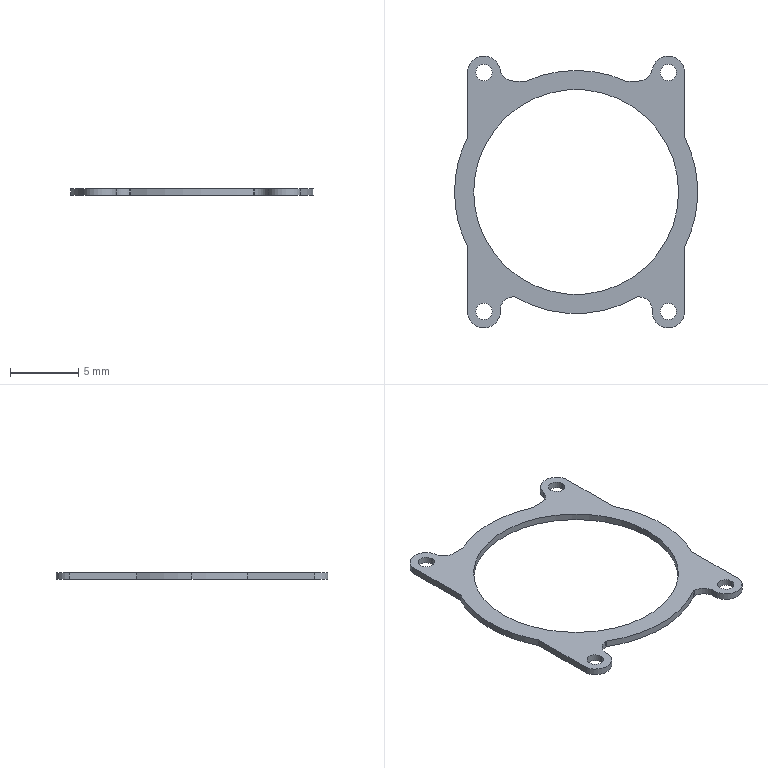Part | SolidWorks | features BaseBody 1, Scale 1 | 1 solid | 35 faces | box 17.8 x 19.9 x 0.5 mm | volume 54.481 mm3 | cylinder 23 | plane 12 | commonest cylinder face diameters 1.2 x8 17.8 x5 2 x4 2.4 x4 15 x2
STEP:
#1=CARTESIAN_POINT('',(7.5,23.098,0.75));
#2=VERTEX_POINT('',#1);
#3=CARTESIAN_POINT('',(-7.5,23.098,0.75));
#4=VERTEX_POINT('',#3);
#5=CARTESIAN_POINT('',(0.,23.098,0.75));
#6=DIRECTION('',(0.,0.,-1.));
#7=DIRECTION('',(-1.,0.,0.));
#8=AXIS2_PLACEMENT_3D('',#5,#6,#7);
#9=CIRCLE('',#8,7.5);
#10=EDGE_CURVE('',#2,#4,#9,.T.);
#11=ORIENTED_EDGE('',*,*,#10,.F.);
#12=CARTESIAN_POINT('',(7.5,23.098,0.25));
#13=VERTEX_POINT('',#12);
#14=CARTESIAN_POINT('',(7.5,23.098,0.75));
#15=DIRECTION('',(0.,0.,-1.));
#16=VECTOR('',#15,1000.);
#17=LINE('',#14,#16);
#18=EDGE_CURVE('',#2,#13,#17,.T.);
#19=ORIENTED_EDGE('',*,*,#18,.T.);
#20=CARTESIAN_POINT('',(-7.5,23.098,0.25));
#21=VERTEX_POINT('',#20);
#22=CARTESIAN_POINT('',(0.,23.098,0.25));
#23=DIRECTION('',(0.,0.,-1.));
#24=DIRECTION('',(-1.,0.,0.));
#25=AXIS2_PLACEMENT_3D('',#22,#23,#24);
#26=CIRCLE('',#25,7.5);
#27=EDGE_CURVE('',#13,#21,#26,.T.);
#28=ORIENTED_EDGE('',*,*,#27,.T.);
#29=CARTESIAN_POINT('',(-7.5,23.098,0.75));
#30=DIRECTION('',(0.,0.,-1.));
#31=VECTOR('',#30,1000.);
#32=LINE('',#29,#31);
#33=EDGE_CURVE('',#4,#21,#32,.T.);
#34=ORIENTED_EDGE('',*,*,#33,.F.);
#35=EDGE_LOOP('',(#11,#19,#28,#34));
#36=FACE_OUTER_BOUND('',#35,.T.);
#37=CARTESIAN_POINT('',(0.,23.098,0.75));
#38=DIRECTION('',(0.,0.,-1.));
#39=DIRECTION('',(-1.,0.,0.));
#40=AXIS2_PLACEMENT_3D('',#37,#38,#39);
#41=CYLINDRICAL_SURFACE('',#40,7.5);
#42=ADVANCED_FACE('',(#36),#41,.F.);
#43=CARTESIAN_POINT('',(-7.926,19.049,0.75));
#44=VERTEX_POINT('',#43);
#45=CARTESIAN_POINT('',(-8.9,23.098,0.75));
#46=VERTEX_POINT('',#45);
#47=CARTESIAN_POINT('',(0.,23.098,0.75));
#48=DIRECTION('',(0.,0.,-1.));
#49=DIRECTION('',(-1.,0.,0.));
#50=AXIS2_PLACEMENT_3D('',#47,#48,#49);
#51=CIRCLE('',#50,8.9);
#52=EDGE_CURVE('',#44,#46,#51,.T.);
#53=ORIENTED_EDGE('',*,*,#52,.T.);
#54=CARTESIAN_POINT('',(-8.9,23.098,0.25));
#55=VERTEX_POINT('',#54);
#56=CARTESIAN_POINT('',(-8.9,23.098,0.75));
#57=DIRECTION('',(0.,0.,-1.));
#58=VECTOR('',#57,1000.);
#59=LINE('',#56,#58);
#60=EDGE_CURVE('',#46,#55,#59,.T.);
#61=ORIENTED_EDGE('',*,*,#60,.T.);
#62=CARTESIAN_POINT('',(-7.926,19.049,0.25));
#63=VERTEX_POINT('',#62);
#64=CARTESIAN_POINT('',(0.,23.098,0.25));
#65=DIRECTION('',(0.,0.,1.));
#66=DIRECTION('',(-1.,0.,0.));
#67=AXIS2_PLACEMENT_3D('',#64,#65,#66);
#68=CIRCLE('',#67,8.9);
#69=EDGE_CURVE('',#55,#63,#68,.T.);
#70=ORIENTED_EDGE('',*,*,#69,.T.);
#71=CARTESIAN_POINT('',(-7.926,19.049,0.75));
#72=DIRECTION('',(0.,0.,1.));
#73=VECTOR('',#72,1000.);
#74=LINE('',#71,#73);
#75=EDGE_CURVE('',#63,#44,#74,.T.);
#76=ORIENTED_EDGE('',*,*,#75,.T.);
#77=EDGE_LOOP('',(#53,#61,#70,#76));
#78=FACE_OUTER_BOUND('',#77,.T.);
#79=CARTESIAN_POINT('',(0.,23.098,0.75));
#80=DIRECTION('',(0.,0.,-1.));
#81=DIRECTION('',(-1.,0.,0.));
#82=AXIS2_PLACEMENT_3D('',#79,#80,#81);
#83=CYLINDRICAL_SURFACE('',#82,8.9);
#84=ADVANCED_FACE('',(#78),#83,.T.);
#85=CARTESIAN_POINT('',(-6.15,14.348,0.25));
#86=VERTEX_POINT('',#85);
#87=CARTESIAN_POINT('',(-7.35,14.348,0.25));
#88=VERTEX_POINT('',#87);
#89=CARTESIAN_POINT('',(-6.75,14.348,0.25));
#90=DIRECTION('',(0.,0.,-1.));
#91=DIRECTION('',(1.,0.,0.));
#92=AXIS2_PLACEMENT_3D('',#89,#90,#91);
#93=CIRCLE('',#92,0.6);
#94=EDGE_CURVE('',#86,#88,#93,.T.);
#95=ORIENTED_EDGE('',*,*,#94,.T.);
#96=CARTESIAN_POINT('',(-7.35,14.348,0.75));
#97=VERTEX_POINT('',#96);
#98=CARTESIAN_POINT('',(-7.35,14.348,0.75));
#99=DIRECTION('',(0.,0.,1.));
#100=VECTOR('',#99,1000.);
#101=LINE('',#98,#100);
#102=EDGE_CURVE('',#88,#97,#101,.T.);
#103=ORIENTED_EDGE('',*,*,#102,.T.);
#104=CARTESIAN_POINT('',(-6.15,14.348,0.75));
#105=VERTEX_POINT('',#104);
#106=CARTESIAN_POINT('',(-6.75,14.348,0.75));
#107=DIRECTION('',(0.,0.,-1.));
#108=DIRECTION('',(1.,0.,0.));
#109=AXIS2_PLACEMENT_3D('',#106,#107,#108);
#110=CIRCLE('',#109,0.6);
#111=EDGE_CURVE('',#105,#97,#110,.T.);
#112=ORIENTED_EDGE('',*,*,#111,.F.);
#113=CARTESIAN_POINT('',(-6.15,14.348,0.75));
#114=DIRECTION('',(0.,0.,1.));
#115=VECTOR('',#114,1000.);
#116=LINE('',#113,#115);
#117=EDGE_CURVE('',#86,#105,#116,.T.);
#118=ORIENTED_EDGE('',*,*,#117,.F.);
#119=EDGE_LOOP('',(#95,#103,#112,#118));
#120=FACE_OUTER_BOUND('',#119,.T.);
#121=CARTESIAN_POINT('',(-6.75,14.348,0.75));
#122=DIRECTION('',(0.,0.,1.));
#123=DIRECTION('',(1.,0.,0.));
#124=AXIS2_PLACEMENT_3D('',#121,#122,#123);
#125=CYLINDRICAL_SURFACE('',#124,0.6);
#126=ADVANCED_FACE('',(#120),#125,.F.);
#127=CARTESIAN_POINT('',(7.35,14.348,0.25));
#128=VERTEX_POINT('',#127);
#129=CARTESIAN_POINT('',(6.15,14.348,0.25));
#130=VERTEX_POINT('',#129);
#131=CARTESIAN_POINT('',(6.75,14.348,0.25));
#132=DIRECTION('',(0.,0.,-1.));
#133=DIRECTION('',(1.,0.,0.));
#134=AXIS2_PLACEMENT_3D('',#131,#132,#133);
#135=CIRCLE('',#134,0.6);
#136=EDGE_CURVE('',#128,#130,#135,.T.);
#137=ORIENTED_EDGE('',*,*,#136,.T.);
#138=CARTESIAN_POINT('',(6.15,14.348,0.75));
#139=VERTEX_POINT('',#138);
#140=CARTESIAN_POINT('',(6.15,14.348,0.75));
#141=DIRECTION('',(0.,0.,1.));
#142=VECTOR('',#141,1000.);
#143=LINE('',#140,#142);
#144=EDGE_CURVE('',#130,#139,#143,.T.);
#145=ORIENTED_EDGE('',*,*,#144,.T.);
#146=CARTESIAN_POINT('',(7.35,14.348,0.75));
#147=VERTEX_POINT('',#146);
#148=CARTESIAN_POINT('',(6.75,14.348,0.75));
#149=DIRECTION('',(0.,0.,-1.));
#150=DIRECTION('',(1.,0.,0.));
#151=AXIS2_PLACEMENT_3D('',#148,#149,#150);
#152=CIRCLE('',#151,0.6);
#153=EDGE_CURVE('',#147,#139,#152,.T.);
#154=ORIENTED_EDGE('',*,*,#153,.F.);
#155=CARTESIAN_POINT('',(7.35,14.348,0.75));
#156=DIRECTION('',(0.,0.,1.));
#157=VECTOR('',#156,1000.);
#158=LINE('',#155,#157);
#159=EDGE_CURVE('',#128,#147,#158,.T.);
#160=ORIENTED_EDGE('',*,*,#159,.F.);
#161=EDGE_LOOP('',(#137,#145,#154,#160));
#162=FACE_OUTER_BOUND('',#161,.T.);
#163=CARTESIAN_POINT('',(6.75,14.348,0.75));
#164=DIRECTION('',(0.,0.,1.));
#165=DIRECTION('',(1.,0.,0.));
#166=AXIS2_PLACEMENT_3D('',#163,#164,#165);
#167=CYLINDRICAL_SURFACE('',#166,0.6);
#168=ADVANCED_FACE('',(#162),#167,.F.);
#169=CARTESIAN_POINT('',(7.35,31.848,0.25));
#170=VERTEX_POINT('',#169);
#171=CARTESIAN_POINT('',(6.15,31.848,0.25));
#172=VERTEX_POINT('',#171);
#173=CARTESIAN_POINT('',(6.75,31.848,0.25));
#174=DIRECTION('',(0.,0.,-1.));
#175=DIRECTION('',(1.,0.,0.));
#176=AXIS2_PLACEMENT_3D('',#173,#174,#175);
#177=CIRCLE('',#176,0.6);
#178=EDGE_CURVE('',#170,#172,#177,.T.);
#179=ORIENTED_EDGE('',*,*,#178,.T.);
#180=CARTESIAN_POINT('',(6.15,31.848,0.75));
#181=VERTEX_POINT('',#180);
#182=CARTESIAN_POINT('',(6.15,31.848,0.75));
#183=DIRECTION('',(0.,0.,1.));
#184=VECTOR('',#183,1000.);
#185=LINE('',#182,#184);
#186=EDGE_CURVE('',#172,#181,#185,.T.);
#187=ORIENTED_EDGE('',*,*,#186,.T.);
#188=CARTESIAN_POINT('',(7.35,31.848,0.75));
#189=VERTEX_POINT('',#188);
#190=CARTESIAN_POINT('',(6.75,31.848,0.75));
#191=DIRECTION('',(0.,0.,-1.));
#192=DIRECTION('',(1.,0.,0.));
#193=AXIS2_PLACEMENT_3D('',#190,#191,#192);
#194=CIRCLE('',#193,0.6);
#195=EDGE_CURVE('',#189,#181,#194,.T.);
#196=ORIENTED_EDGE('',*,*,#195,.F.);
#197=CARTESIAN_POINT('',(7.35,31.848,0.75));
#198=DIRECTION('',(0.,0.,1.));
#199=VECTOR('',#198,1000.);
#200=LINE('',#197,#199);
#201=EDGE_CURVE('',#170,#189,#200,.T.);
#202=ORIENTED_EDGE('',*,*,#201,.F.);
#203=EDGE_LOOP('',(#179,#187,#196,#202));
#204=FACE_OUTER_BOUND('',#203,.T.);
#205=CARTESIAN_POINT('',(6.75,31.848,0.75));
#206=DIRECTION('',(0.,0.,1.));
#207=DIRECTION('',(1.,0.,0.));
#208=AXIS2_PLACEMENT_3D('',#205,#206,#207);
#209=CYLINDRICAL_SURFACE('',#208,0.6);
#210=ADVANCED_FACE('',(#204),#209,.F.);
#211=CARTESIAN_POINT('',(-6.15,31.848,0.25));
#212=VERTEX_POINT('',#211);
#213=CARTESIAN_POINT('',(-7.35,31.848,0.25));
#214=VERTEX_POINT('',#213);
#215=CARTESIAN_POINT('',(-6.75,31.848,0.25));
#216=DIRECTION('',(0.,0.,-1.));
#217=DIRECTION('',(1.,0.,0.));
#218=AXIS2_PLACEMENT_3D('',#215,#216,#217);
#219=CIRCLE('',#218,0.6);
#220=EDGE_CURVE('',#212,#214,#219,.T.);
#221=ORIENTED_EDGE('',*,*,#220,.T.);
#222=CARTESIAN_POINT('',(-7.35,31.848,0.75));
#223=VERTEX_POINT('',#222);
#224=CARTESIAN_POINT('',(-7.35,31.848,0.75));
#225=DIRECTION('',(0.,0.,1.));
#226=VECTOR('',#225,1000.);
#227=LINE('',#224,#226);
#228=EDGE_CURVE('',#214,#223,#227,.T.);
#229=ORIENTED_EDGE('',*,*,#228,.T.);
#230=CARTESIAN_POINT('',(-6.15,31.848,0.75));
#231=VERTEX_POINT('',#230);
#232=CARTESIAN_POINT('',(-6.75,31.848,0.75));
#233=DIRECTION('',(0.,0.,-1.));
#234=DIRECTION('',(1.,0.,0.));
#235=AXIS2_PLACEMENT_3D('',#232,#233,#234);
#236=CIRCLE('',#235,0.6);
#237=EDGE_CURVE('',#231,#223,#236,.T.);
#238=ORIENTED_EDGE('',*,*,#237,.F.);
#239=CARTESIAN_POINT('',(-6.15,31.848,0.75));
#240=DIRECTION('',(0.,0.,1.));
#241=VECTOR('',#240,1000.);
#242=LINE('',#239,#241);
#243=EDGE_CURVE('',#212,#231,#242,.T.);
#244=ORIENTED_EDGE('',*,*,#243,.F.);
#245=EDGE_LOOP('',(#221,#229,#238,#244));
#246=FACE_OUTER_BOUND('',#245,.T.);
#247=CARTESIAN_POINT('',(-6.75,31.848,0.75));
#248=DIRECTION('',(0.,0.,1.));
#249=DIRECTION('',(1.,0.,0.));
#250=AXIS2_PLACEMENT_3D('',#247,#248,#249);
#251=CYLINDRICAL_SURFACE('',#250,0.6);
#252=ADVANCED_FACE('',(#246),#251,.F.);
#253=CARTESIAN_POINT('',(0.,23.098,0.25));
#254=DIRECTION('',(0.,0.,-1.));
#255=DIRECTION('',(-1.,0.,0.));
#256=AXIS2_PLACEMENT_3D('',#253,#254,#255);
#257=CIRCLE('',#256,7.5);
#258=EDGE_CURVE('',#21,#13,#257,.T.);
#259=ORIENTED_EDGE('',*,*,#258,.F.);
#260=ORIENTED_EDGE('',*,*,#27,.F.);
#261=EDGE_LOOP('',(#259,#260));
#262=FACE_BOUND('',#261,.T.);
#263=CARTESIAN_POINT('',(-7.926,32.088,0.25));
#264=VERTEX_POINT('',#263);
#265=CARTESIAN_POINT('',(-7.926,27.146,0.25));
#266=VERTEX_POINT('',#265);
#267=CARTESIAN_POINT('',(-7.926,23.098,0.25));
#268=DIRECTION('',(0.,-1.,0.));
#269=VECTOR('',#268,1000.);
#270=LINE('',#267,#269);
#271=EDGE_CURVE('',#264,#266,#270,.T.);
#272=ORIENTED_EDGE('',*,*,#271,.F.);
#273=CARTESIAN_POINT('',(-5.574,32.088,0.25));
#274=VERTEX_POINT('',#273);
#275=CARTESIAN_POINT('',(-6.75,31.848,0.25));
#276=DIRECTION('',(0.,0.,1.));
#277=DIRECTION('',(-1.,0.,0.));
#278=AXIS2_PLACEMENT_3D('',#275,#276,#277);
#279=CIRCLE('',#278,1.2);
#280=EDGE_CURVE('',#274,#264,#279,.T.);
#281=ORIENTED_EDGE('',*,*,#280,.F.);
#282=CARTESIAN_POINT('',(-4.583,31.223,0.25));
#283=VERTEX_POINT('',#282);
#284=CARTESIAN_POINT('',(-4.583,32.223,0.25));
#285=DIRECTION('',(0.,0.,-1.));
#286=DIRECTION('',(-1.,0.,0.));
#287=AXIS2_PLACEMENT_3D('',#284,#285,#286);
#288=CIRCLE('',#287,1.);
#289=EDGE_CURVE('',#283,#274,#288,.T.);
#290=ORIENTED_EDGE('',*,*,#289,.F.);
#291=CARTESIAN_POINT('',(-3.632,31.223,0.25));
#292=VERTEX_POINT('',#291);
#293=CARTESIAN_POINT('',(0.,31.223,0.25));
#294=DIRECTION('',(-1.,0.,0.));
#295=VECTOR('',#294,1000.);
#296=LINE('',#293,#295);
#297=EDGE_CURVE('',#292,#283,#296,.T.);
#298=ORIENTED_EDGE('',*,*,#297,.F.);
#299=CARTESIAN_POINT('',(3.632,31.223,0.25));
#300=VERTEX_POINT('',#299);
#301=CARTESIAN_POINT('',(0.,23.098,0.25));
#302=DIRECTION('',(0.,0.,1.));
#303=DIRECTION('',(-1.,0.,0.));
#304=AXIS2_PLACEMENT_3D('',#301,#302,#303);
#305=CIRCLE('',#304,8.9);
#306=EDGE_CURVE('',#300,#292,#305,.T.);
#307=ORIENTED_EDGE('',*,*,#306,.F.);
#308=CARTESIAN_POINT('',(4.583,31.223,0.25));
#309=VERTEX_POINT('',#308);
#310=CARTESIAN_POINT('',(0.,31.223,0.25));
#311=DIRECTION('',(-1.,0.,0.));
#312=VECTOR('',#311,1000.);
#313=LINE('',#310,#312);
#314=EDGE_CURVE('',#309,#300,#313,.T.);
#315=ORIENTED_EDGE('',*,*,#314,.F.);
#316=CARTESIAN_POINT('',(5.574,32.088,0.25));
#317=VERTEX_POINT('',#316);
#318=CARTESIAN_POINT('',(4.583,32.223,0.25));
#319=DIRECTION('',(0.,0.,-1.));
#320=DIRECTION('',(-1.,0.,0.));
#321=AXIS2_PLACEMENT_3D('',#318,#319,#320);
#322=CIRCLE('',#321,1.);
#323=EDGE_CURVE('',#317,#309,#322,.T.);
#324=ORIENTED_EDGE('',*,*,#323,.F.);
#325=CARTESIAN_POINT('',(7.926,32.088,0.25));
#326=VERTEX_POINT('',#325);
#327=CARTESIAN_POINT('',(6.75,31.848,0.25));
#328=DIRECTION('',(0.,0.,1.));
#329=DIRECTION('',(-1.,0.,0.));
#330=AXIS2_PLACEMENT_3D('',#327,#328,#329);
#331=CIRCLE('',#330,1.2);
#332=EDGE_CURVE('',#326,#317,#331,.T.);
#333=ORIENTED_EDGE('',*,*,#332,.F.);
#334=CARTESIAN_POINT('',(7.926,27.146,0.25));
#335=VERTEX_POINT('',#334);
#336=CARTESIAN_POINT('',(7.926,23.098,0.25));
#337=DIRECTION('',(0.,1.,0.));
#338=VECTOR('',#337,1000.);
#339=LINE('',#336,#338);
#340=EDGE_CURVE('',#335,#326,#339,.T.);
#341=ORIENTED_EDGE('',*,*,#340,.F.);
#342=CARTESIAN_POINT('',(7.926,19.049,0.25));
#343=VERTEX_POINT('',#342);
#344=CARTESIAN_POINT('',(0.,23.098,0.25));
#345=DIRECTION('',(0.,0.,1.));
#346=DIRECTION('',(-1.,0.,0.));
#347=AXIS2_PLACEMENT_3D('',#344,#345,#346);
#348=CIRCLE('',#347,8.9);
#349=EDGE_CURVE('',#343,#335,#348,.T.);
#350=ORIENTED_EDGE('',*,*,#349,.F.);
#351=CARTESIAN_POINT('',(7.926,14.108,0.25));
#352=VERTEX_POINT('',#351);
#353=CARTESIAN_POINT('',(7.926,23.098,0.25));
#354=DIRECTION('',(0.,1.,0.));
#355=VECTOR('',#354,1000.);
#356=LINE('',#353,#355);
#357=EDGE_CURVE('',#352,#343,#356,.T.);
#358=ORIENTED_EDGE('',*,*,#357,.F.);
#359=CARTESIAN_POINT('',(5.574,14.108,0.25));
#360=VERTEX_POINT('',#359);
#361=CARTESIAN_POINT('',(6.75,14.348,0.25));
#362=DIRECTION('',(0.,0.,1.));
#363=DIRECTION('',(-1.,0.,0.));
#364=AXIS2_PLACEMENT_3D('',#361,#362,#363);
#365=CIRCLE('',#364,1.2);
#366=EDGE_CURVE('',#360,#352,#365,.T.);
#367=ORIENTED_EDGE('',*,*,#366,.F.);
#368=CARTESIAN_POINT('',(5.574,14.423,0.25));
#369=VERTEX_POINT('',#368);
#370=CARTESIAN_POINT('',(5.574,23.098,0.25));
#371=DIRECTION('',(0.,-1.,0.));
#372=VECTOR('',#371,1000.);
#373=LINE('',#370,#372);
#374=EDGE_CURVE('',#369,#360,#373,.T.);
#375=ORIENTED_EDGE('',*,*,#374,.F.);
#376=CARTESIAN_POINT('',(4.574,15.423,0.25));
#377=VERTEX_POINT('',#376);
#378=CARTESIAN_POINT('',(4.574,14.423,0.25));
#379=DIRECTION('',(0.,0.,-1.));
#380=DIRECTION('',(1.,0.,0.));
#381=AXIS2_PLACEMENT_3D('',#378,#379,#380);
#382=CIRCLE('',#381,1.);
#383=EDGE_CURVE('',#377,#369,#382,.T.);
#384=ORIENTED_EDGE('',*,*,#383,.F.);
#385=CARTESIAN_POINT('',(4.506,15.423,0.25));
#386=VERTEX_POINT('',#385);
#387=CARTESIAN_POINT('',(0.,15.423,0.25));
#388=DIRECTION('',(1.,0.,0.));
#389=VECTOR('',#388,1000.);
#390=LINE('',#387,#389);
#391=EDGE_CURVE('',#386,#377,#390,.T.);
#392=ORIENTED_EDGE('',*,*,#391,.F.);
#393=CARTESIAN_POINT('',(-4.506,15.423,0.25));
#394=VERTEX_POINT('',#393);
#395=CARTESIAN_POINT('',(0.,23.098,0.25));
#396=DIRECTION('',(0.,0.,1.));
#397=DIRECTION('',(-1.,0.,0.));
#398=AXIS2_PLACEMENT_3D('',#395,#396,#397);
#399=CIRCLE('',#398,8.9);
#400=EDGE_CURVE('',#394,#386,#399,.T.);
#401=ORIENTED_EDGE('',*,*,#400,.F.);
#402=CARTESIAN_POINT('',(-4.574,15.423,0.25));
#403=VERTEX_POINT('',#402);
#404=CARTESIAN_POINT('',(0.,15.423,0.25));
#405=DIRECTION('',(1.,0.,0.));
#406=VECTOR('',#405,1000.);
#407=LINE('',#404,#406);
#408=EDGE_CURVE('',#403,#394,#407,.T.);
#409=ORIENTED_EDGE('',*,*,#408,.F.);
#410=CARTESIAN_POINT('',(-5.574,14.423,0.25));
#411=VERTEX_POINT('',#410);
#412=CARTESIAN_POINT('',(-4.574,14.423,0.25));
#413=DIRECTION('',(0.,0.,-1.));
#414=DIRECTION('',(1.,0.,0.));
#415=AXIS2_PLACEMENT_3D('',#412,#413,#414);
#416=CIRCLE('',#415,1.);
#417=EDGE_CURVE('',#411,#403,#416,.T.);
#418=ORIENTED_EDGE('',*,*,#417,.F.);
#419=CARTESIAN_POINT('',(-5.574,14.108,0.25));
#420=VERTEX_POINT('',#419);
#421=CARTESIAN_POINT('',(-5.574,23.098,0.25));
#422=DIRECTION('',(0.,1.,0.));
#423=VECTOR('',#422,1000.);
#424=LINE('',#421,#423);
#425=EDGE_CURVE('',#420,#411,#424,.T.);
#426=ORIENTED_EDGE('',*,*,#425,.F.);
#427=CARTESIAN_POINT('',(-7.926,14.108,0.25));
#428=VERTEX_POINT('',#427);
#429=CARTESIAN_POINT('',(-6.75,14.348,0.25));
#430=DIRECTION('',(0.,0.,1.));
#431=DIRECTION('',(-1.,0.,0.));
#432=AXIS2_PLACEMENT_3D('',#429,#430,#431);
#433=CIRCLE('',#432,1.2);
#434=EDGE_CURVE('',#428,#420,#433,.T.);
#435=ORIENTED_EDGE('',*,*,#434,.F.);
#436=CARTESIAN_POINT('',(-7.926,23.098,0.25));
#437=DIRECTION('',(0.,-1.,0.));
#438=VECTOR('',#437,1000.);
#439=LINE('',#436,#438);
#440=EDGE_CURVE('',#63,#428,#439,.T.);
#441=ORIENTED_EDGE('',*,*,#440,.F.);
#442=ORIENTED_EDGE('',*,*,#69,.F.);
#443=CARTESIAN_POINT('',(0.,23.098,0.25));
#444=DIRECTION('',(0.,0.,1.));
#445=DIRECTION('',(-1.,0.,0.));
#446=AXIS2_PLACEMENT_3D('',#443,#444,#445);
#447=CIRCLE('',#446,8.9);
#448=EDGE_CURVE('',#266,#55,#447,.T.);
#449=ORIENTED_EDGE('',*,*,#448,.F.);
#450=EDGE_LOOP('',(#272,#281,#290,#298,#307,#315,#324,#333,#341,#350,#358,#367,#375,#384,#392,#401,#409,#418,#426,#435,#441,#442,#449));
#451=FACE_OUTER_BOUND('',#450,.T.);
#452=ORIENTED_EDGE('',*,*,#94,.F.);
#453=CARTESIAN_POINT('',(-6.75,14.348,0.25));
#454=DIRECTION('',(0.,0.,-1.));
#455=DIRECTION('',(1.,0.,0.));
#456=AXIS2_PLACEMENT_3D('',#453,#454,#455);
#457=CIRCLE('',#456,0.6);
#458=EDGE_CURVE('',#88,#86,#457,.T.);
#459=ORIENTED_EDGE('',*,*,#458,.F.);
#460=EDGE_LOOP('',(#452,#459));
#461=FACE_BOUND('',#460,.T.);
#462=ORIENTED_EDGE('',*,*,#136,.F.);
#463=CARTESIAN_POINT('',(6.75,14.348,0.25));
#464=DIRECTION('',(0.,0.,-1.));
#465=DIRECTION('',(1.,0.,0.));
#466=AXIS2_PLACEMENT_3D('',#463,#464,#465);
#467=CIRCLE('',#466,0.6);
#468=EDGE_CURVE('',#130,#128,#467,.T.);
#469=ORIENTED_EDGE('',*,*,#468,.F.);
#470=EDGE_LOOP('',(#462,#469));
#471=FACE_BOUND('',#470,.T.);
#472=ORIENTED_EDGE('',*,*,#178,.F.);
#473=CARTESIAN_POINT('',(6.75,31.848,0.25));
#474=DIRECTION('',(0.,0.,-1.));
#475=DIRECTION('',(1.,0.,0.));
#476=AXIS2_PLACEMENT_3D('',#473,#474,#475);
#477=CIRCLE('',#476,0.6);
#478=EDGE_CURVE('',#172,#170,#477,.T.);
#479=ORIENTED_EDGE('',*,*,#478,.F.);
#480=EDGE_LOOP('',(#472,#479));
#481=FACE_BOUND('',#480,.T.);
#482=ORIENTED_EDGE('',*,*,#220,.F.);
#483=CARTESIAN_POINT('',(-6.75,31.848,0.25));
#484=DIRECTION('',(0.,0.,-1.));
#485=DIRECTION('',(1.,0.,0.));
#486=AXIS2_PLACEMENT_3D('',#483,#484,#485);
#487=CIRCLE('',#486,0.6);
#488=EDGE_CURVE('',#214,#212,#487,.T.);
#489=ORIENTED_EDGE('',*,*,#488,.F.);
#490=EDGE_LOOP('',(#482,#489));
#491=FACE_BOUND('',#490,.T.);
#492=CARTESIAN_POINT('',(0.,23.098,0.25));
#493=DIRECTION('',(0.,0.,1.));
#494=DIRECTION('',(1.,0.,0.));
#495=AXIS2_PLACEMENT_3D('',#492,#493,#494);
#496=PLANE('',#495);
#497=ADVANCED_FACE('',(#262,#451,#461,#471,#481,#491),#496,.F.);
#498=ORIENTED_EDGE('',*,*,#18,.F.);
#499=CARTESIAN_POINT('',(0.,23.098,0.75));
#500=DIRECTION('',(0.,0.,-1.));
#501=DIRECTION('',(-1.,0.,0.));
#502=AXIS2_PLACEMENT_3D('',#499,#500,#501);
#503=CIRCLE('',#502,7.5);
#504=EDGE_CURVE('',#4,#2,#503,.T.);
#505=ORIENTED_EDGE('',*,*,#504,.F.);
#506=ORIENTED_EDGE('',*,*,#33,.T.);
#507=ORIENTED_EDGE('',*,*,#258,.T.);
#508=EDGE_LOOP('',(#498,#505,#506,#507));
#509=FACE_OUTER_BOUND('',#508,.T.);
#510=CARTESIAN_POINT('',(0.,23.098,0.75));
#511=DIRECTION('',(0.,0.,-1.));
#512=DIRECTION('',(-1.,0.,0.));
#513=AXIS2_PLACEMENT_3D('',#510,#511,#512);
#514=CYLINDRICAL_SURFACE('',#513,7.5);
#515=ADVANCED_FACE('',(#509),#514,.F.);
#516=ORIENTED_EDGE('',*,*,#60,.F.);
#517=CARTESIAN_POINT('',(-7.926,27.146,0.75));
#518=VERTEX_POINT('',#517);
#519=CARTESIAN_POINT('',(0.,23.098,0.75));
#520=DIRECTION('',(0.,0.,-1.));
#521=DIRECTION('',(-1.,0.,0.));
#522=AXIS2_PLACEMENT_3D('',#519,#520,#521);
#523=CIRCLE('',#522,8.9);
#524=EDGE_CURVE('',#46,#518,#523,.T.);
#525=ORIENTED_EDGE('',*,*,#524,.T.);
#526=CARTESIAN_POINT('',(-7.926,27.146,0.75));
#527=DIRECTION('',(0.,0.,-1.));
#528=VECTOR('',#527,1000.);
#529=LINE('',#526,#528);
#530=EDGE_CURVE('',#518,#266,#529,.T.);
#531=ORIENTED_EDGE('',*,*,#530,.T.);
#532=ORIENTED_EDGE('',*,*,#448,.T.);
#533=EDGE_LOOP('',(#516,#525,#531,#532));
#534=FACE_OUTER_BOUND('',#533,.T.);
#535=CARTESIAN_POINT('',(0.,23.098,0.75));
#536=DIRECTION('',(0.,0.,-1.));
#537=DIRECTION('',(-1.,0.,0.));
#538=AXIS2_PLACEMENT_3D('',#535,#536,#537);
#539=CYLINDRICAL_SURFACE('',#538,8.9);
#540=ADVANCED_FACE('',(#534),#539,.T.);
#541=ORIENTED_EDGE('',*,*,#530,.F.);
#542=CARTESIAN_POINT('',(-7.926,32.088,0.75));
#543=VERTEX_POINT('',#542);
#544=CARTESIAN_POINT('',(-7.926,32.088,0.75));
#545=DIRECTION('',(0.,-1.,0.));
#546=VECTOR('',#545,1000.);
#547=LINE('',#544,#546);
#548=EDGE_CURVE('',#543,#518,#547,.T.);
#549=ORIENTED_EDGE('',*,*,#548,.F.);
#550=CARTESIAN_POINT('',(-7.926,32.088,0.75));
#551=DIRECTION('',(0.,0.,1.));
#552=VECTOR('',#551,1000.);
#553=LINE('',#550,#552);
#554=EDGE_CURVE('',#264,#543,#553,.T.);
#555=ORIENTED_EDGE('',*,*,#554,.F.);
#556=ORIENTED_EDGE('',*,*,#271,.T.);
#557=EDGE_LOOP('',(#541,#549,#555,#556));
#558=FACE_OUTER_BOUND('',#557,.T.);
#559=CARTESIAN_POINT('',(-7.926,32.088,0.75));
#560=DIRECTION('',(1.,0.,0.));
#561=DIRECTION('',(0.,1.,0.));
#562=AXIS2_PLACEMENT_3D('',#559,#560,#561);
#563=PLANE('',#562);
#564=ADVANCED_FACE('',(#558),#563,.F.);
#565=CARTESIAN_POINT('',(-5.574,32.088,0.75));
#566=VERTEX_POINT('',#565);
#567=CARTESIAN_POINT('',(-6.75,31.848,0.75));
#568=DIRECTION('',(0.,0.,-1.));
#569=DIRECTION('',(-1.,0.,0.));
#570=AXIS2_PLACEMENT_3D('',#567,#568,#569);
#571=CIRCLE('',#570,1.2);
#572=EDGE_CURVE('',#543,#566,#571,.T.);
#573=ORIENTED_EDGE('',*,*,#572,.T.);
#574=CARTESIAN_POINT('',(-5.574,32.088,0.75));
#575=DIRECTION('',(0.,0.,-1.));
#576=VECTOR('',#575,1000.);
#577=LINE('',#574,#576);
#578=EDGE_CURVE('',#566,#274,#577,.T.);
#579=ORIENTED_EDGE('',*,*,#578,.T.);
#580=ORIENTED_EDGE('',*,*,#280,.T.);
#581=ORIENTED_EDGE('',*,*,#554,.T.);
#582=EDGE_LOOP('',(#573,#579,#580,#581));
#583=FACE_OUTER_BOUND('',#582,.T.);
#584=CARTESIAN_POINT('',(-6.75,31.848,0.75));
#585=DIRECTION('',(0.,0.,-1.));
#586=DIRECTION('',(-1.,0.,0.));
#587=AXIS2_PLACEMENT_3D('',#584,#585,#586);
#588=CYLINDRICAL_SURFACE('',#587,1.2);
#589=ADVANCED_FACE('',(#583),#588,.T.);
#590=CARTESIAN_POINT('',(-4.583,31.223,0.75));
#591=VERTEX_POINT('',#590);
#592=CARTESIAN_POINT('',(-4.583,31.223,0.75));
#593=DIRECTION('',(0.,0.,1.));
#594=VECTOR('',#593,1000.);
#595=LINE('',#592,#594);
#596=EDGE_CURVE('',#283,#591,#595,.T.);
#597=ORIENTED_EDGE('',*,*,#596,.F.);
#598=ORIENTED_EDGE('',*,*,#289,.T.);
#599=ORIENTED_EDGE('',*,*,#578,.F.);
#600=CARTESIAN_POINT('',(-4.583,32.223,0.75));
#601=DIRECTION('',(0.,0.,-1.));
#602=DIRECTION('',(-1.,0.,0.));
#603=AXIS2_PLACEMENT_3D('',#600,#601,#602);
#604=CIRCLE('',#603,1.);
#605=EDGE_CURVE('',#591,#566,#604,.T.);
#606=ORIENTED_EDGE('',*,*,#605,.F.);
#607=EDGE_LOOP('',(#597,#598,#599,#606));
#608=FACE_OUTER_BOUND('',#607,.T.);
#609=CARTESIAN_POINT('',(-4.583,32.223,0.75));
#610=DIRECTION('',(0.,0.,-1.));
#611=DIRECTION('',(-1.,0.,0.));
#612=AXIS2_PLACEMENT_3D('',#609,#610,#611);
#613=CYLINDRICAL_SURFACE('',#612,1.);
#614=ADVANCED_FACE('',(#608),#613,.F.);
#615=ORIENTED_EDGE('',*,*,#596,.T.);
#616=CARTESIAN_POINT('',(-3.632,31.223,0.75));
#617=VERTEX_POINT('',#616);
#618=CARTESIAN_POINT('',(-3.632,31.223,0.75));
#619=DIRECTION('',(-1.,0.,0.));
#620=VECTOR('',#619,1000.);
#621=LINE('',#618,#620);
#622=EDGE_CURVE('',#617,#591,#621,.T.);
#623=ORIENTED_EDGE('',*,*,#622,.F.);
#624=CARTESIAN_POINT('',(-3.632,31.223,0.75));
#625=DIRECTION('',(0.,0.,1.));
#626=VECTOR('',#625,1000.);
#627=LINE('',#624,#626);
#628=EDGE_CURVE('',#292,#617,#627,.T.);
#629=ORIENTED_EDGE('',*,*,#628,.F.);
#630=ORIENTED_EDGE('',*,*,#297,.T.);
#631=EDGE_LOOP('',(#615,#623,#629,#630));
#632=FACE_OUTER_BOUND('',#631,.T.);
#633=CARTESIAN_POINT('',(-3.632,31.223,0.75));
#634=DIRECTION('',(0.,-1.,0.));
#635=DIRECTION('',(0.,0.,-1.));
#636=AXIS2_PLACEMENT_3D('',#633,#634,#635);
#637=PLANE('',#636);
#638=ADVANCED_FACE('',(#632),#637,.F.);
#639=CARTESIAN_POINT('',(3.632,31.223,0.75));
#640=VERTEX_POINT('',#639);
#641=CARTESIAN_POINT('',(0.,23.098,0.75));
#642=DIRECTION('',(0.,0.,-1.));
#643=DIRECTION('',(-1.,0.,0.));
#644=AXIS2_PLACEMENT_3D('',#641,#642,#643);
#645=CIRCLE('',#644,8.9);
#646=EDGE_CURVE('',#617,#640,#645,.T.);
#647=ORIENTED_EDGE('',*,*,#646,.T.);
#648=CARTESIAN_POINT('',(3.632,31.223,0.75));
#649=DIRECTION('',(0.,0.,-1.));
#650=VECTOR('',#649,1000.);
#651=LINE('',#648,#650);
#652=EDGE_CURVE('',#640,#300,#651,.T.);
#653=ORIENTED_EDGE('',*,*,#652,.T.);
#654=ORIENTED_EDGE('',*,*,#306,.T.);
#655=ORIENTED_EDGE('',*,*,#628,.T.);
#656=EDGE_LOOP('',(#647,#653,#654,#655));
#657=FACE_OUTER_BOUND('',#656,.T.);
#658=CARTESIAN_POINT('',(0.,23.098,0.75));
#659=DIRECTION('',(0.,0.,-1.));
#660=DIRECTION('',(-1.,0.,0.));
#661=AXIS2_PLACEMENT_3D('',#658,#659,#660);
#662=CYLINDRICAL_SURFACE('',#661,8.9);
#663=ADVANCED_FACE('',(#657),#662,.T.);
#664=CARTESIAN_POINT('',(4.583,31.223,0.75));
#665=VERTEX_POINT('',#664);
#666=CARTESIAN_POINT('',(4.583,31.223,0.75));
#667=DIRECTION('',(0.,0.,1.));
#668=VECTOR('',#667,1000.);
#669=LINE('',#666,#668);
#670=EDGE_CURVE('',#309,#665,#669,.T.);
#671=ORIENTED_EDGE('',*,*,#670,.F.);
#672=ORIENTED_EDGE('',*,*,#314,.T.);
#673=ORIENTED_EDGE('',*,*,#652,.F.);
#674=CARTESIAN_POINT('',(5.574,31.223,0.75));
#675=DIRECTION('',(-1.,0.,0.));
#676=VECTOR('',#675,1000.);
#677=LINE('',#674,#676);
#678=EDGE_CURVE('',#665,#640,#677,.T.);
#679=ORIENTED_EDGE('',*,*,#678,.F.);
#680=EDGE_LOOP('',(#671,#672,#673,#679));
#681=FACE_OUTER_BOUND('',#680,.T.);
#682=CARTESIAN_POINT('',(5.574,31.223,0.75));
#683=DIRECTION('',(0.,-1.,0.));
#684=DIRECTION('',(1.,0.,0.));
#685=AXIS2_PLACEMENT_3D('',#682,#683,#684);
#686=PLANE('',#685);
#687=ADVANCED_FACE('',(#681),#686,.F.);
#688=CARTESIAN_POINT('',(5.574,32.088,0.75));
#689=VERTEX_POINT('',#688);
#690=CARTESIAN_POINT('',(5.574,32.088,0.75));
#691=DIRECTION('',(0.,0.,1.));
#692=VECTOR('',#691,1000.);
#693=LINE('',#690,#692);
#694=EDGE_CURVE('',#317,#689,#693,.T.);
#695=ORIENTED_EDGE('',*,*,#694,.F.);
#696=ORIENTED_EDGE('',*,*,#323,.T.);
#697=ORIENTED_EDGE('',*,*,#670,.T.);
#698=CARTESIAN_POINT('',(4.583,32.223,0.75));
#699=DIRECTION('',(0.,0.,-1.));
#700=DIRECTION('',(-1.,0.,0.));
#701=AXIS2_PLACEMENT_3D('',#698,#699,#700);
#702=CIRCLE('',#701,1.);
#703=EDGE_CURVE('',#689,#665,#702,.T.);
#704=ORIENTED_EDGE('',*,*,#703,.F.);
#705=EDGE_LOOP('',(#695,#696,#697,#704));
#706=FACE_OUTER_BOUND('',#705,.T.);
#707=CARTESIAN_POINT('',(4.583,32.223,0.75));
#708=DIRECTION('',(0.,0.,-1.));
#709=DIRECTION('',(-1.,0.,0.));
#710=AXIS2_PLACEMENT_3D('',#707,#708,#709);
#711=CYLINDRICAL_SURFACE('',#710,1.);
#712=ADVANCED_FACE('',(#706),#711,.F.);
#713=CARTESIAN_POINT('',(7.926,32.088,0.75));
#714=VERTEX_POINT('',#713);
#715=CARTESIAN_POINT('',(6.75,31.848,0.75));
#716=DIRECTION('',(0.,0.,-1.));
#717=DIRECTION('',(-1.,0.,0.));
#718=AXIS2_PLACEMENT_3D('',#715,#716,#717);
#719=CIRCLE('',#718,1.2);
#720=EDGE_CURVE('',#689,#714,#719,.T.);
#721=ORIENTED_EDGE('',*,*,#720,.T.);
#722=CARTESIAN_POINT('',(7.926,32.088,0.75));
#723=DIRECTION('',(0.,0.,-1.));
#724=VECTOR('',#723,1000.);
#725=LINE('',#722,#724);
#726=EDGE_CURVE('',#714,#326,#725,.T.);
#727=ORIENTED_EDGE('',*,*,#726,.T.);
#728=ORIENTED_EDGE('',*,*,#332,.T.);
#729=ORIENTED_EDGE('',*,*,#694,.T.);
#730=EDGE_LOOP('',(#721,#727,#728,#729));
#731=FACE_OUTER_BOUND('',#730,.T.);
#732=CARTESIAN_POINT('',(6.75,31.848,0.75));
#733=DIRECTION('',(0.,0.,-1.));
#734=DIRECTION('',(-1.,0.,0.));
#735=AXIS2_PLACEMENT_3D('',#732,#733,#734);
#736=CYLINDRICAL_SURFACE('',#735,1.2);
#737=ADVANCED_FACE('',(#731),#736,.T.);
#738=ORIENTED_EDGE('',*,*,#726,.F.);
#739=CARTESIAN_POINT('',(7.926,27.146,0.75));
#740=VERTEX_POINT('',#739);
#741=CARTESIAN_POINT('',(7.926,27.146,0.75));
#742=DIRECTION('',(0.,1.,0.));
#743=VECTOR('',#742,1000.);
#744=LINE('',#741,#743);
#745=EDGE_CURVE('',#740,#714,#744,.T.);
#746=ORIENTED_EDGE('',*,*,#745,.F.);
#747=CARTESIAN_POINT('',(7.926,27.146,0.75));
#748=DIRECTION('',(0.,0.,1.));
#749=VECTOR('',#748,1000.);
#750=LINE('',#747,#749);
#751=EDGE_CURVE('',#335,#740,#750,.T.);
#752=ORIENTED_EDGE('',*,*,#751,.F.);
#753=ORIENTED_EDGE('',*,*,#340,.T.);
#754=EDGE_LOOP('',(#738,#746,#752,#753));
#755=FACE_OUTER_BOUND('',#754,.T.);
#756=CARTESIAN_POINT('',(7.926,27.146,0.75));
#757=DIRECTION('',(-1.,0.,0.));
#758=DIRECTION('',(0.,0.,1.));
#759=AXIS2_PLACEMENT_3D('',#756,#757,#758);
#760=PLANE('',#759);
#761=ADVANCED_FACE('',(#755),#760,.F.);
#762=CARTESIAN_POINT('',(7.926,19.049,0.75));
#763=VERTEX_POINT('',#762);
#764=CARTESIAN_POINT('',(0.,23.098,0.75));
#765=DIRECTION('',(0.,0.,-1.));
#766=DIRECTION('',(-1.,0.,0.));
#767=AXIS2_PLACEMENT_3D('',#764,#765,#766);
#768=CIRCLE('',#767,8.9);
#769=EDGE_CURVE('',#740,#763,#768,.T.);
#770=ORIENTED_EDGE('',*,*,#769,.T.);
#771=CARTESIAN_POINT('',(7.926,19.049,0.75));
#772=DIRECTION('',(0.,0.,-1.));
#773=VECTOR('',#772,1000.);
#774=LINE('',#771,#773);
#775=EDGE_CURVE('',#763,#343,#774,.T.);
#776=ORIENTED_EDGE('',*,*,#775,.T.);
#777=ORIENTED_EDGE('',*,*,#349,.T.);
#778=ORIENTED_EDGE('',*,*,#751,.T.);
#779=EDGE_LOOP('',(#770,#776,#777,#778));
#780=FACE_OUTER_BOUND('',#779,.T.);
#781=CARTESIAN_POINT('',(0.,23.098,0.75));
#782=DIRECTION('',(0.,0.,-1.));
#783=DIRECTION('',(-1.,0.,0.));
#784=AXIS2_PLACEMENT_3D('',#781,#782,#783);
#785=CYLINDRICAL_SURFACE('',#784,8.9);
#786=ADVANCED_FACE('',(#780),#785,.T.);
#787=ORIENTED_EDGE('',*,*,#775,.F.);
#788=CARTESIAN_POINT('',(7.926,14.108,0.75));
#789=VERTEX_POINT('',#788);
#790=CARTESIAN_POINT('',(7.926,14.108,0.75));
#791=DIRECTION('',(0.,1.,0.));
#792=VECTOR('',#791,1000.);
#793=LINE('',#790,#792);
#794=EDGE_CURVE('',#789,#763,#793,.T.);
#795=ORIENTED_EDGE('',*,*,#794,.F.);
#796=CARTESIAN_POINT('',(7.926,14.108,0.75));
#797=DIRECTION('',(0.,0.,1.));
#798=VECTOR('',#797,1000.);
#799=LINE('',#796,#798);
#800=EDGE_CURVE('',#352,#789,#799,.T.);
#801=ORIENTED_EDGE('',*,*,#800,.F.);
#802=ORIENTED_EDGE('',*,*,#357,.T.);
#803=EDGE_LOOP('',(#787,#795,#801,#802));
#804=FACE_OUTER_BOUND('',#803,.T.);
#805=CARTESIAN_POINT('',(7.926,14.108,0.75));
#806=DIRECTION('',(-1.,0.,0.));
#807=DIRECTION('',(0.,0.,1.));
#808=AXIS2_PLACEMENT_3D('',#805,#806,#807);
#809=PLANE('',#808);
#810=ADVANCED_FACE('',(#804),#809,.F.);
#811=CARTESIAN_POINT('',(5.574,14.108,0.75));
#812=VERTEX_POINT('',#811);
#813=CARTESIAN_POINT('',(6.75,14.348,0.75));
#814=DIRECTION('',(0.,0.,-1.));
#815=DIRECTION('',(-1.,0.,0.));
#816=AXIS2_PLACEMENT_3D('',#813,#814,#815);
#817=CIRCLE('',#816,1.2);
#818=EDGE_CURVE('',#789,#812,#817,.T.);
#819=ORIENTED_EDGE('',*,*,#818,.T.);
#820=CARTESIAN_POINT('',(5.574,14.108,0.75));
#821=DIRECTION('',(0.,0.,-1.));
#822=VECTOR('',#821,1000.);
#823=LINE('',#820,#822);
#824=EDGE_CURVE('',#812,#360,#823,.T.);
#825=ORIENTED_EDGE('',*,*,#824,.T.);
#826=ORIENTED_EDGE('',*,*,#366,.T.);
#827=ORIENTED_EDGE('',*,*,#800,.T.);
#828=EDGE_LOOP('',(#819,#825,#826,#827));
#829=FACE_OUTER_BOUND('',#828,.T.);
#830=CARTESIAN_POINT('',(6.75,14.348,0.75));
#831=DIRECTION('',(0.,0.,-1.));
#832=DIRECTION('',(-1.,0.,0.));
#833=AXIS2_PLACEMENT_3D('',#830,#831,#832);
#834=CYLINDRICAL_SURFACE('',#833,1.2);
#835=ADVANCED_FACE('',(#829),#834,.T.);
#836=CARTESIAN_POINT('',(5.574,14.423,0.75));
#837=VERTEX_POINT('',#836);
#838=CARTESIAN_POINT('',(5.574,14.423,0.75));
#839=DIRECTION('',(0.,0.,1.));
#840=VECTOR('',#839,1000.);
#841=LINE('',#838,#840);
#842=EDGE_CURVE('',#369,#837,#841,.T.);
#843=ORIENTED_EDGE('',*,*,#842,.F.);
#844=ORIENTED_EDGE('',*,*,#374,.T.);
#845=ORIENTED_EDGE('',*,*,#824,.F.);
#846=CARTESIAN_POINT('',(5.574,15.423,0.75));
#847=DIRECTION('',(0.,-1.,0.));
#848=VECTOR('',#847,1000.);
#849=LINE('',#846,#848);
#850=EDGE_CURVE('',#837,#812,#849,.T.);
#851=ORIENTED_EDGE('',*,*,#850,.F.);
#852=EDGE_LOOP('',(#843,#844,#845,#851));
#853=FACE_OUTER_BOUND('',#852,.T.);
#854=CARTESIAN_POINT('',(5.574,15.423,0.75));
#855=DIRECTION('',(1.,0.,0.));
#856=DIRECTION('',(0.,0.,-1.));
#857=AXIS2_PLACEMENT_3D('',#854,#855,#856);
#858=PLANE('',#857);
#859=ADVANCED_FACE('',(#853),#858,.F.);
#860=CARTESIAN_POINT('',(4.574,15.423,0.75));
#861=VERTEX_POINT('',#860);
#862=CARTESIAN_POINT('',(4.574,15.423,0.75));
#863=DIRECTION('',(0.,0.,1.));
#864=VECTOR('',#863,1000.);
#865=LINE('',#862,#864);
#866=EDGE_CURVE('',#377,#861,#865,.T.);
#867=ORIENTED_EDGE('',*,*,#866,.F.);
#868=ORIENTED_EDGE('',*,*,#383,.T.);
#869=ORIENTED_EDGE('',*,*,#842,.T.);
#870=CARTESIAN_POINT('',(4.574,14.423,0.75));
#871=DIRECTION('',(0.,0.,-1.));
#872=DIRECTION('',(1.,0.,0.));
#873=AXIS2_PLACEMENT_3D('',#870,#871,#872);
#874=CIRCLE('',#873,1.);
#875=EDGE_CURVE('',#861,#837,#874,.T.);
#876=ORIENTED_EDGE('',*,*,#875,.F.);
#877=EDGE_LOOP('',(#867,#868,#869,#876));
#878=FACE_OUTER_BOUND('',#877,.T.);
#879=CARTESIAN_POINT('',(4.574,14.423,0.75));
#880=DIRECTION('',(0.,0.,1.));
#881=DIRECTION('',(1.,0.,0.));
#882=AXIS2_PLACEMENT_3D('',#879,#880,#881);
#883=CYLINDRICAL_SURFACE('',#882,1.);
#884=ADVANCED_FACE('',(#878),#883,.F.);
#885=ORIENTED_EDGE('',*,*,#866,.T.);
#886=CARTESIAN_POINT('',(4.506,15.423,0.75));
#887=VERTEX_POINT('',#886);
#888=CARTESIAN_POINT('',(4.506,15.423,0.75));
#889=DIRECTION('',(1.,0.,0.));
#890=VECTOR('',#889,1000.);
#891=LINE('',#888,#890);
#892=EDGE_CURVE('',#887,#861,#891,.T.);
#893=ORIENTED_EDGE('',*,*,#892,.F.);
#894=CARTESIAN_POINT('',(4.506,15.423,0.75));
#895=DIRECTION('',(0.,0.,1.));
#896=VECTOR('',#895,1000.);
#897=LINE('',#894,#896);
#898=EDGE_CURVE('',#386,#887,#897,.T.);
#899=ORIENTED_EDGE('',*,*,#898,.F.);
#900=ORIENTED_EDGE('',*,*,#391,.T.);
#901=EDGE_LOOP('',(#885,#893,#899,#900));
#902=FACE_OUTER_BOUND('',#901,.T.);
#903=CARTESIAN_POINT('',(4.506,15.423,0.75));
#904=DIRECTION('',(0.,1.,0.));
#905=DIRECTION('',(-1.,0.,0.));
#906=AXIS2_PLACEMENT_3D('',#903,#904,#905);
#907=PLANE('',#906);
#908=ADVANCED_FACE('',(#902),#907,.F.);
#909=CARTESIAN_POINT('',(-4.506,15.423,0.75));
#910=VERTEX_POINT('',#909);
#911=CARTESIAN_POINT('',(0.,23.098,0.75));
#912=DIRECTION('',(0.,0.,-1.));
#913=DIRECTION('',(-1.,0.,0.));
#914=AXIS2_PLACEMENT_3D('',#911,#912,#913);
#915=CIRCLE('',#914,8.9);
#916=EDGE_CURVE('',#887,#910,#915,.T.);
#917=ORIENTED_EDGE('',*,*,#916,.T.);
#918=CARTESIAN_POINT('',(-4.506,15.423,0.75));
#919=DIRECTION('',(0.,0.,-1.));
#920=VECTOR('',#919,1000.);
#921=LINE('',#918,#920);
#922=EDGE_CURVE('',#910,#394,#921,.T.);
#923=ORIENTED_EDGE('',*,*,#922,.T.);
#924=ORIENTED_EDGE('',*,*,#400,.T.);
#925=ORIENTED_EDGE('',*,*,#898,.T.);
#926=EDGE_LOOP('',(#917,#923,#924,#925));
#927=FACE_OUTER_BOUND('',#926,.T.);
#928=CARTESIAN_POINT('',(0.,23.098,0.75));
#929=DIRECTION('',(0.,0.,-1.));
#930=DIRECTION('',(-1.,0.,0.));
#931=AXIS2_PLACEMENT_3D('',#928,#929,#930);
#932=CYLINDRICAL_SURFACE('',#931,8.9);
#933=ADVANCED_FACE('',(#927),#932,.T.);
#934=CARTESIAN_POINT('',(-4.574,15.423,0.75));
#935=VERTEX_POINT('',#934);
#936=CARTESIAN_POINT('',(-4.574,15.423,0.75));
#937=DIRECTION('',(0.,0.,1.));
#938=VECTOR('',#937,1000.);
#939=LINE('',#936,#938);
#940=EDGE_CURVE('',#403,#935,#939,.T.);
#941=ORIENTED_EDGE('',*,*,#940,.F.);
#942=ORIENTED_EDGE('',*,*,#408,.T.);
#943=ORIENTED_EDGE('',*,*,#922,.F.);
#944=CARTESIAN_POINT('',(-5.574,15.423,0.75));
#945=DIRECTION('',(1.,0.,0.));
#946=VECTOR('',#945,1000.);
#947=LINE('',#944,#946);
#948=EDGE_CURVE('',#935,#910,#947,.T.);
#949=ORIENTED_EDGE('',*,*,#948,.F.);
#950=EDGE_LOOP('',(#941,#942,#943,#949));
#951=FACE_OUTER_BOUND('',#950,.T.);
#952=CARTESIAN_POINT('',(-5.574,15.423,0.75));
#953=DIRECTION('',(0.,1.,0.));
#954=DIRECTION('',(-1.,0.,0.));
#955=AXIS2_PLACEMENT_3D('',#952,#953,#954);
#956=PLANE('',#955);
#957=ADVANCED_FACE('',(#951),#956,.F.);
#958=CARTESIAN_POINT('',(-5.574,14.423,0.75));
#959=VERTEX_POINT('',#958);
#960=CARTESIAN_POINT('',(-5.574,14.423,0.75));
#961=DIRECTION('',(0.,0.,1.));
#962=VECTOR('',#961,1000.);
#963=LINE('',#960,#962);
#964=EDGE_CURVE('',#411,#959,#963,.T.);
#965=ORIENTED_EDGE('',*,*,#964,.F.);
#966=ORIENTED_EDGE('',*,*,#417,.T.);
#967=ORIENTED_EDGE('',*,*,#940,.T.);
#968=CARTESIAN_POINT('',(-4.574,14.423,0.75));
#969=DIRECTION('',(0.,0.,-1.));
#970=DIRECTION('',(1.,0.,0.));
#971=AXIS2_PLACEMENT_3D('',#968,#969,#970);
#972=CIRCLE('',#971,1.);
#973=EDGE_CURVE('',#959,#935,#972,.T.);
#974=ORIENTED_EDGE('',*,*,#973,.F.);
#975=EDGE_LOOP('',(#965,#966,#967,#974));
#976=FACE_OUTER_BOUND('',#975,.T.);
#977=CARTESIAN_POINT('',(-4.574,14.423,0.75));
#978=DIRECTION('',(0.,0.,1.));
#979=DIRECTION('',(1.,0.,0.));
#980=AXIS2_PLACEMENT_3D('',#977,#978,#979);
#981=CYLINDRICAL_SURFACE('',#980,1.);
#982=ADVANCED_FACE('',(#976),#981,.F.);
#983=ORIENTED_EDGE('',*,*,#964,.T.);
#984=CARTESIAN_POINT('',(-5.574,14.108,0.75));
#985=VERTEX_POINT('',#984);
#986=CARTESIAN_POINT('',(-5.574,14.108,0.75));
#987=DIRECTION('',(0.,1.,0.));
#988=VECTOR('',#987,1000.);
#989=LINE('',#986,#988);
#990=EDGE_CURVE('',#985,#959,#989,.T.);
#991=ORIENTED_EDGE('',*,*,#990,.F.);
#992=CARTESIAN_POINT('',(-5.574,14.108,0.75));
#993=DIRECTION('',(0.,0.,1.));
#994=VECTOR('',#993,1000.);
#995=LINE('',#992,#994);
#996=EDGE_CURVE('',#420,#985,#995,.T.);
#997=ORIENTED_EDGE('',*,*,#996,.F.);
#998=ORIENTED_EDGE('',*,*,#425,.T.);
#999=EDGE_LOOP('',(#983,#991,#997,#998));
#1000=FACE_OUTER_BOUND('',#999,.T.);
#1001=CARTESIAN_POINT('',(-5.574,14.108,0.75));
#1002=DIRECTION('',(-1.,0.,0.));
#1003=DIRECTION('',(0.,0.,1.));
#1004=AXIS2_PLACEMENT_3D('',#1001,#1002,#1003);
#1005=PLANE('',#1004);
#1006=ADVANCED_FACE('',(#1000),#1005,.F.);
#1007=CARTESIAN_POINT('',(-7.926,14.108,0.75));
#1008=VERTEX_POINT('',#1007);
#1009=CARTESIAN_POINT('',(-6.75,14.348,0.75));
#1010=DIRECTION('',(0.,0.,-1.));
#1011=DIRECTION('',(-1.,0.,0.));
#1012=AXIS2_PLACEMENT_3D('',#1009,#1010,#1011);
#1013=CIRCLE('',#1012,1.2);
#1014=EDGE_CURVE('',#985,#1008,#1013,.T.);
#1015=ORIENTED_EDGE('',*,*,#1014,.T.);
#1016=CARTESIAN_POINT('',(-7.926,14.108,0.75));
#1017=DIRECTION('',(0.,0.,-1.));
#1018=VECTOR('',#1017,1000.);
#1019=LINE('',#1016,#1018);
#1020=EDGE_CURVE('',#1008,#428,#1019,.T.);
#1021=ORIENTED_EDGE('',*,*,#1020,.T.);
#1022=ORIENTED_EDGE('',*,*,#434,.T.);
#1023=ORIENTED_EDGE('',*,*,#996,.T.);
#1024=EDGE_LOOP('',(#1015,#1021,#1022,#1023));
#1025=FACE_OUTER_BOUND('',#1024,.T.);
#1026=CARTESIAN_POINT('',(-6.75,14.348,0.75));
#1027=DIRECTION('',(0.,0.,-1.));
#1028=DIRECTION('',(-1.,0.,0.));
#1029=AXIS2_PLACEMENT_3D('',#1026,#1027,#1028);
#1030=CYLINDRICAL_SURFACE('',#1029,1.2);
#1031=ADVANCED_FACE('',(#1025),#1030,.T.);
#1032=ORIENTED_EDGE('',*,*,#1020,.F.);
#1033=CARTESIAN_POINT('',(-7.926,19.049,0.75));
#1034=DIRECTION('',(0.,-1.,0.));
#1035=VECTOR('',#1034,1000.);
#1036=LINE('',#1033,#1035);
#1037=EDGE_CURVE('',#44,#1008,#1036,.T.);
#1038=ORIENTED_EDGE('',*,*,#1037,.F.);
#1039=ORIENTED_EDGE('',*,*,#75,.F.);
#1040=ORIENTED_EDGE('',*,*,#440,.T.);
#1041=EDGE_LOOP('',(#1032,#1038,#1039,#1040));
#1042=FACE_OUTER_BOUND('',#1041,.T.);
#1043=CARTESIAN_POINT('',(-7.926,19.049,0.75));
#1044=DIRECTION('',(1.,0.,0.));
#1045=DIRECTION('',(0.,0.,-1.));
#1046=AXIS2_PLACEMENT_3D('',#1043,#1044,#1045);
#1047=PLANE('',#1046);
#1048=ADVANCED_FACE('',(#1042),#1047,.F.);
#1049=ORIENTED_EDGE('',*,*,#102,.F.);
#1050=ORIENTED_EDGE('',*,*,#458,.T.);
#1051=ORIENTED_EDGE('',*,*,#117,.T.);
#1052=CARTESIAN_POINT('',(-6.75,14.348,0.75));
#1053=DIRECTION('',(0.,0.,-1.));
#1054=DIRECTION('',(1.,0.,0.));
#1055=AXIS2_PLACEMENT_3D('',#1052,#1053,#1054);
#1056=CIRCLE('',#1055,0.6);
#1057=EDGE_CURVE('',#97,#105,#1056,.T.);
#1058=ORIENTED_EDGE('',*,*,#1057,.F.);
#1059=EDGE_LOOP('',(#1049,#1050,#1051,#1058));
#1060=FACE_OUTER_BOUND('',#1059,.T.);
#1061=CARTESIAN_POINT('',(-6.75,14.348,0.75));
#1062=DIRECTION('',(0.,0.,1.));
#1063=DIRECTION('',(1.,0.,0.));
#1064=AXIS2_PLACEMENT_3D('',#1061,#1062,#1063);
#1065=CYLINDRICAL_SURFACE('',#1064,0.6);
#1066=ADVANCED_FACE('',(#1060),#1065,.F.);
#1067=ORIENTED_EDGE('',*,*,#144,.F.);
#1068=ORIENTED_EDGE('',*,*,#468,.T.);
#1069=ORIENTED_EDGE('',*,*,#159,.T.);
#1070=CARTESIAN_POINT('',(6.75,14.348,0.75));
#1071=DIRECTION('',(0.,0.,-1.));
#1072=DIRECTION('',(1.,0.,0.));
#1073=AXIS2_PLACEMENT_3D('',#1070,#1071,#1072);
#1074=CIRCLE('',#1073,0.6);
#1075=EDGE_CURVE('',#139,#147,#1074,.T.);
#1076=ORIENTED_EDGE('',*,*,#1075,.F.);
#1077=EDGE_LOOP('',(#1067,#1068,#1069,#1076));
#1078=FACE_OUTER_BOUND('',#1077,.T.);
#1079=CARTESIAN_POINT('',(6.75,14.348,0.75));
#1080=DIRECTION('',(0.,0.,1.));
#1081=DIRECTION('',(1.,0.,0.));
#1082=AXIS2_PLACEMENT_3D('',#1079,#1080,#1081);
#1083=CYLINDRICAL_SURFACE('',#1082,0.6);
#1084=ADVANCED_FACE('',(#1078),#1083,.F.);
#1085=ORIENTED_EDGE('',*,*,#186,.F.);
#1086=ORIENTED_EDGE('',*,*,#478,.T.);
#1087=ORIENTED_EDGE('',*,*,#201,.T.);
#1088=CARTESIAN_POINT('',(6.75,31.848,0.75));
#1089=DIRECTION('',(0.,0.,-1.));
#1090=DIRECTION('',(1.,0.,0.));
#1091=AXIS2_PLACEMENT_3D('',#1088,#1089,#1090);
#1092=CIRCLE('',#1091,0.6);
#1093=EDGE_CURVE('',#181,#189,#1092,.T.);
#1094=ORIENTED_EDGE('',*,*,#1093,.F.);
#1095=EDGE_LOOP('',(#1085,#1086,#1087,#1094));
#1096=FACE_OUTER_BOUND('',#1095,.T.);
#1097=CARTESIAN_POINT('',(6.75,31.848,0.75));
#1098=DIRECTION('',(0.,0.,1.));
#1099=DIRECTION('',(1.,0.,0.));
#1100=AXIS2_PLACEMENT_3D('',#1097,#1098,#1099);
#1101=CYLINDRICAL_SURFACE('',#1100,0.6);
#1102=ADVANCED_FACE('',(#1096),#1101,.F.);
#1103=ORIENTED_EDGE('',*,*,#228,.F.);
#1104=ORIENTED_EDGE('',*,*,#488,.T.);
#1105=ORIENTED_EDGE('',*,*,#243,.T.);
#1106=CARTESIAN_POINT('',(-6.75,31.848,0.75));
#1107=DIRECTION('',(0.,0.,-1.));
#1108=DIRECTION('',(1.,0.,0.));
#1109=AXIS2_PLACEMENT_3D('',#1106,#1107,#1108);
#1110=CIRCLE('',#1109,0.6);
#1111=EDGE_CURVE('',#223,#231,#1110,.T.);
#1112=ORIENTED_EDGE('',*,*,#1111,.F.);
#1113=EDGE_LOOP('',(#1103,#1104,#1105,#1112));
#1114=FACE_OUTER_BOUND('',#1113,.T.);
#1115=CARTESIAN_POINT('',(-6.75,31.848,0.75));
#1116=DIRECTION('',(0.,0.,1.));
#1117=DIRECTION('',(1.,0.,0.));
#1118=AXIS2_PLACEMENT_3D('',#1115,#1116,#1117);
#1119=CYLINDRICAL_SURFACE('',#1118,0.6);
#1120=ADVANCED_FACE('',(#1114),#1119,.F.);
#1121=ORIENTED_EDGE('',*,*,#504,.T.);
#1122=ORIENTED_EDGE('',*,*,#10,.T.);
#1123=EDGE_LOOP('',(#1121,#1122));
#1124=FACE_BOUND('',#1123,.T.);
#1125=ORIENTED_EDGE('',*,*,#572,.F.);
#1126=ORIENTED_EDGE('',*,*,#548,.T.);
#1127=ORIENTED_EDGE('',*,*,#524,.F.);
#1128=ORIENTED_EDGE('',*,*,#52,.F.);
#1129=ORIENTED_EDGE('',*,*,#1037,.T.);
#1130=ORIENTED_EDGE('',*,*,#1014,.F.);
#1131=ORIENTED_EDGE('',*,*,#990,.T.);
#1132=ORIENTED_EDGE('',*,*,#973,.T.);
#1133=ORIENTED_EDGE('',*,*,#948,.T.);
#1134=ORIENTED_EDGE('',*,*,#916,.F.);
#1135=ORIENTED_EDGE('',*,*,#892,.T.);
#1136=ORIENTED_EDGE('',*,*,#875,.T.);
#1137=ORIENTED_EDGE('',*,*,#850,.T.);
#1138=ORIENTED_EDGE('',*,*,#818,.F.);
#1139=ORIENTED_EDGE('',*,*,#794,.T.);
#1140=ORIENTED_EDGE('',*,*,#769,.F.);
#1141=ORIENTED_EDGE('',*,*,#745,.T.);
#1142=ORIENTED_EDGE('',*,*,#720,.F.);
#1143=ORIENTED_EDGE('',*,*,#703,.T.);
#1144=ORIENTED_EDGE('',*,*,#678,.T.);
#1145=ORIENTED_EDGE('',*,*,#646,.F.);
#1146=ORIENTED_EDGE('',*,*,#622,.T.);
#1147=ORIENTED_EDGE('',*,*,#605,.T.);
#1148=EDGE_LOOP('',(#1125,#1126,#1127,#1128,#1129,#1130,#1131,#1132,#1133,#1134,#1135,#1136,#1137,#1138,#1139,#1140,#1141,#1142,#1143,#1144,#1145,#1146,#1147));
#1149=FACE_OUTER_BOUND('',#1148,.T.);
#1150=ORIENTED_EDGE('',*,*,#111,.T.);
#1151=ORIENTED_EDGE('',*,*,#1057,.T.);
#1152=EDGE_LOOP('',(#1150,#1151));
#1153=FACE_BOUND('',#1152,.T.);
#1154=ORIENTED_EDGE('',*,*,#153,.T.);
#1155=ORIENTED_EDGE('',*,*,#1075,.T.);
#1156=EDGE_LOOP('',(#1154,#1155));
#1157=FACE_BOUND('',#1156,.T.);
#1158=ORIENTED_EDGE('',*,*,#195,.T.);
#1159=ORIENTED_EDGE('',*,*,#1093,.T.);
#1160=EDGE_LOOP('',(#1158,#1159));
#1161=FACE_BOUND('',#1160,.T.);
#1162=ORIENTED_EDGE('',*,*,#237,.T.);
#1163=ORIENTED_EDGE('',*,*,#1111,.T.);
#1164=EDGE_LOOP('',(#1162,#1163));
#1165=FACE_BOUND('',#1164,.T.);
#1166=CARTESIAN_POINT('',(0.,23.098,0.75));
#1167=DIRECTION('',(0.,0.,1.));
#1168=DIRECTION('',(1.,0.,0.));
#1169=AXIS2_PLACEMENT_3D('',#1166,#1167,#1168);
#1170=PLANE('',#1169);
#1171=ADVANCED_FACE('',(#1124,#1149,#1153,#1157,#1161,#1165),#1170,.T.);
#1172=CLOSED_SHELL('',(#42,#84,#126,#168,#210,#252,#497,#515,#540,#564,#589,#614,#638,#663,#687,#712,#737,#761,#786,#810,#835,#859,#884,#908,#933,#957,#982,#1006,#1031,#1048,#1066,#1084,#1102,#1120,#1171));
#1173=MANIFOLD_SOLID_BREP('',#1172);
#1174=CARTESIAN_POINT('',(0.,0.,0.));
#1175=DIRECTION('',(0.,0.,1.));
#1176=DIRECTION('',(1.,0.,0.));
#1177=AXIS2_PLACEMENT_3D('',#1174,#1175,#1176);
#1178=(LENGTH_UNIT()NAMED_UNIT(*)SI_UNIT(.MILLI.,.METRE.));
#1179=UNCERTAINTY_MEASURE_WITH_UNIT(LENGTH_MEASURE(0.00001),#1178,'','');
#1180=(NAMED_UNIT(*)PLANE_ANGLE_UNIT()SI_UNIT($,.RADIAN.));
#1181=(NAMED_UNIT(*)SI_UNIT($,.STERADIAN.)SOLID_ANGLE_UNIT());
#1182=(GEOMETRIC_REPRESENTATION_CONTEXT(3)GLOBAL_UNCERTAINTY_ASSIGNED_CONTEXT((#1179))GLOBAL_UNIT_ASSIGNED_CONTEXT((#1178,#1180,#1181))REPRESENTATION_CONTEXT('',''));
#1183=ADVANCED_BREP_SHAPE_REPRESENTATION('',(#1173,#1177),#1182);